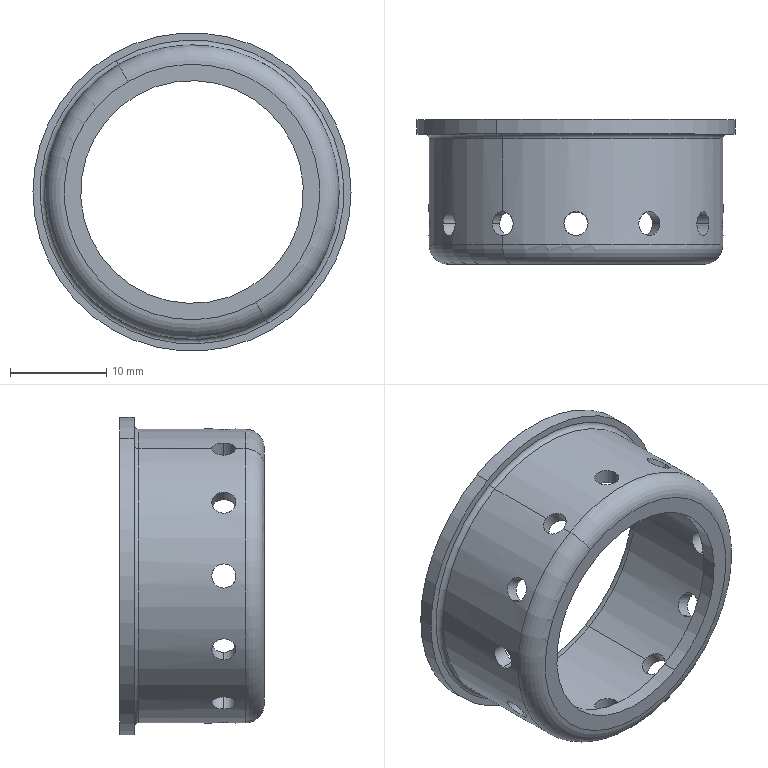Part | SolidWorks | features BaseBody 1 | 1 solid | 46 faces | box 33 x 15 x 33 mm | volume 2295 mm3 | cylinder 32 | torus 8 | plane 4 | cone 2 | commonest cylinder face diameters 2.5 x24 23.1 x2 27.5 x2 30.5 x2 33 x2